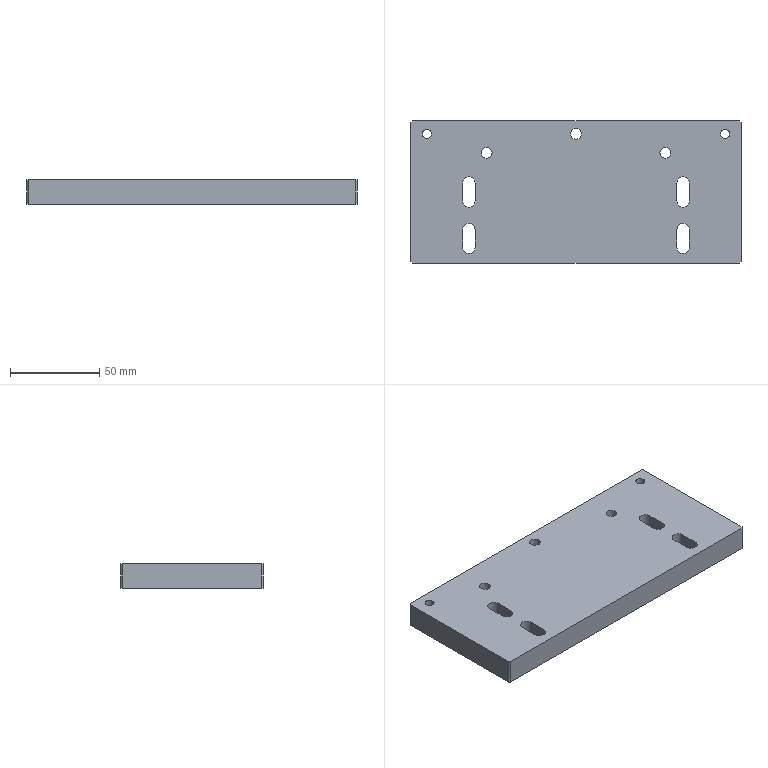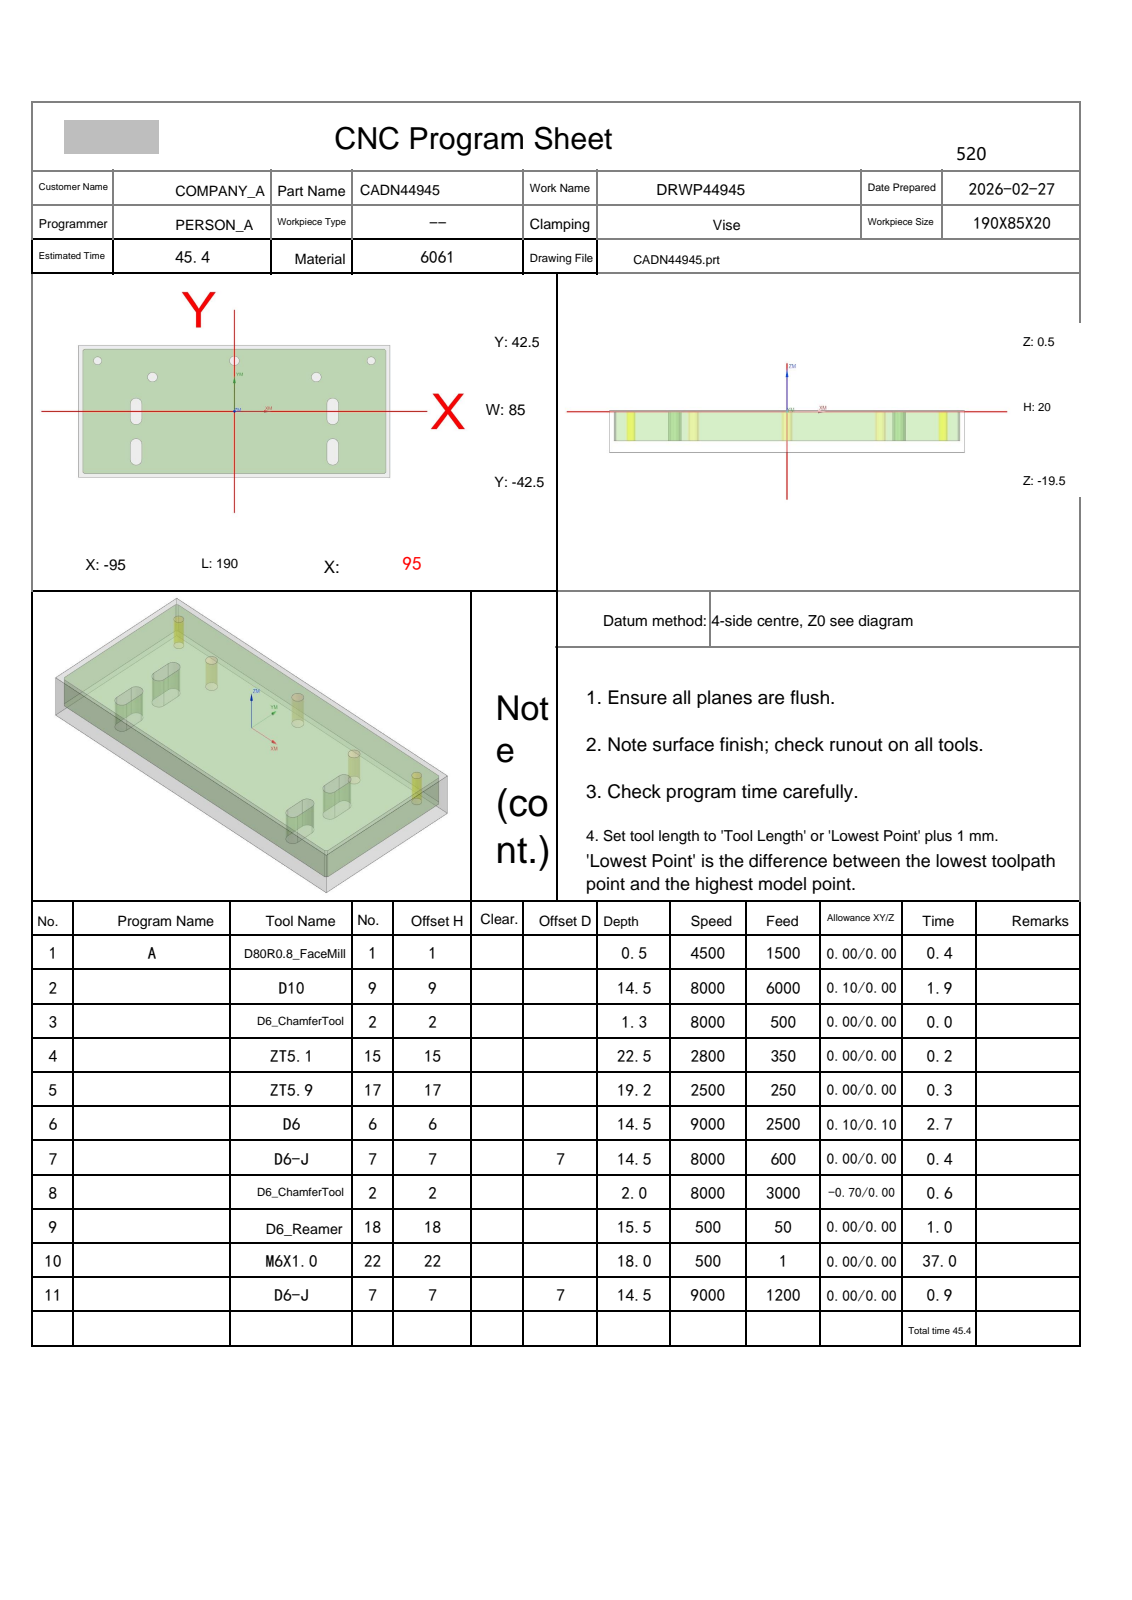NC program | NX | posted by the shop | part box 185 x 80 x 14 mm
Lines 439 to 1302 of 2772:
N6 T06 M06
(D6  D=6. R=0. H=06 ce=0.10 di=0.10)
G00 G90 G54 X-59.6 Y-26. M03 S9000
G43 H06 Z50.
M08
Z.5
G01 Y-21. Z.456 F2500.
G03 X-59.778 Y-20.667 Z.452 I-.4 J0.0
X-60. Y-20.6 Z.45 I-.222 J-.333
X-60.4 Y-21. Z.445 I0.0 J-.4
G01 Y-31. Z.357
G03 X-60. Y-31.4 Z.351 I.4 J0.0
X-59.6 Y-31. Z.345 I0.0 J.4
G01 Y-21. Z.257
G03 X-59.778 Y-20.667 Z.254 I-.4 J0.0
X-60. Y-20.6 Z.252 I-.222 J-.333
X-60.4 Y-21. Z.246 I0.0 J-.4
G01 Y-31. Z.158
G03 X-60. Y-31.4 Z.152 I.4 J0.0
X-59.6 Y-31. Z.147 I0.0 J.4
G01 Y-21. Z.059
G03 X-59.778 Y-20.667 Z.055 I-.4 J0.0
X-60. Y-20.6 Z.053 I-.222 J-.333
X-60.4 Y-21. Z.048 I0.0 J-.4
G01 Y-31. Z-.041
G03 X-60. Y-31.4 Z-.046 I.4 J0.0
X-59.6 Y-31. Z-.052 I0.0 J.4
G01 Y-21. Z-.14
G03 X-59.778 Y-20.667 Z-.143 I-.4 J0.0
X-60. Y-20.6 Z-.146 I-.222 J-.333
X-60.4 Y-21. Z-.151 I0.0 J-.4
G01 Y-31. Z-.239
G03 X-60. Y-31.4 Z-.245 I.4 J0.0
X-59.6 Y-31. Z-.25 I0.0 J.4
G01 Y-21. Z-.339
G03 X-59.778 Y-20.667 Z-.342 I-.4 J0.0
X-60. Y-20.6 Z-.344 I-.222 J-.333
X-60.4 Y-21. Z-.35 I0.0 J-.4
G01 Y-31. Z-.438
G03 X-60. Y-31.4 Z-.443 I.4 J0.0
X-59.6 Y-31. Z-.449 I0.0 J.4
G01 Y-21. Z-.537
G03 X-59.778 Y-20.667 Z-.541 I-.4 J0.0
X-60. Y-20.6 Z-.543 I-.222 J-.333
X-60.4 Y-21. Z-.548 I0.0 J-.4
G01 Y-31. Z-.637
G03 X-60. Y-31.4 Z-.642 I.4 J0.0
X-59.6 Y-31. Z-.648 I0.0 J.4
G01 Y-21. Z-.736
G03 X-59.778 Y-20.667 Z-.739 I-.4 J0.0
X-60. Y-20.6 Z-.741 I-.222 J-.333
X-60.4 Y-21. Z-.747 I0.0 J-.4
G01 Y-31. Z-.835
G03 X-60. Y-31.4 Z-.841 I.4 J0.0
X-59.6 Y-31. Z-.846 I0.0 J.4
G01 Y-21. Z-.935
G03 X-59.778 Y-20.667 Z-.938 I-.4 J0.0
X-60. Y-20.6 Z-.94 I-.222 J-.333
X-60.4 Y-21. Z-.946 I0.0 J-.4
G01 Y-31. Z-1.034
G03 X-60. Y-31.4 Z-1.039 I.4 J0.0
X-59.6 Y-31. Z-1.045 I0.0 J.4
G01 Y-21. Z-1.133
G03 X-59.778 Y-20.667 Z-1.137 I-.4 J0.0
X-60. Y-20.6 Z-1.139 I-.222 J-.333
X-60.4 Y-21. Z-1.144 I0.0 J-.4
G01 Y-31. Z-1.232
G03 X-60. Y-31.4 Z-1.238 I.4 J0.0
X-59.6 Y-31. Z-1.244 I0.0 J.4
G01 Y-21. Z-1.332
G03 X-59.778 Y-20.667 Z-1.335 I-.4 J0.0
X-60. Y-20.6 Z-1.337 I-.222 J-.333
X-60.4 Y-21. Z-1.343 I0.0 J-.4
G01 Y-31. Z-1.431
G03 X-60. Y-31.4 Z-1.437 I.4 J0.0
X-59.6 Y-31. Z-1.442 I0.0 J.4
G01 Y-21. Z-1.53
G03 X-59.778 Y-20.667 Z-1.534 I-.4 J0.0
X-60. Y-20.6 Z-1.536 I-.222 J-.333
X-60.4 Y-21. Z-1.542 I0.0 J-.4
G01 Y-31. Z-1.63
G03 X-60. Y-31.4 Z-1.635 I.4 J0.0
X-59.6 Y-31. Z-1.641 I0.0 J.4
G01 Y-21. Z-1.729
G03 X-59.778 Y-20.667 Z-1.733 I-.4 J0.0
X-60. Y-20.6 Z-1.735 I-.222 J-.333
X-60.4 Y-21. Z-1.74 I0.0 J-.4
G01 Y-31. Z-1.828
G03 X-60. Y-31.4 Z-1.834 I.4 J0.0
X-59.6 Y-31. Z-1.839 I0.0 J.4
G01 Y-21. Z-1.928
G03 X-59.778 Y-20.667 Z-1.931 I-.4 J0.0
X-60. Y-20.6 Z-1.933 I-.222 J-.333
X-60.4 Y-21. Z-1.939 I0.0 J-.4
G01 Y-31. Z-2.027
G03 X-60. Y-31.4 Z-2.033 I.4 J0.0
X-59.6 Y-31. Z-2.038 I0.0 J.4
G01 Y-21. Z-2.126
G03 X-59.778 Y-20.667 Z-2.13 I-.4 J0.0
X-60. Y-20.6 Z-2.132 I-.222 J-.333
X-60.4 Y-21. Z-2.137 I0.0 J-.4
G01 Y-31. Z-2.226
G03 X-60. Y-31.4 Z-2.231 I.4 J0.0
X-59.6 Y-31. Z-2.237 I0.0 J.4
G01 Y-21. Z-2.325
G03 X-59.778 Y-20.667 Z-2.328 I-.4 J0.0
X-60. Y-20.6 Z-2.33 I-.222 J-.333
X-60.4 Y-21. Z-2.336 I0.0 J-.4
G01 Y-31. Z-2.424
G03 X-60. Y-31.4 Z-2.43 I.4 J0.0
X-59.6 Y-31. Z-2.435 I0.0 J.4
G01 Y-21. Z-2.524
G03 X-59.778 Y-20.667 Z-2.527 I-.4 J0.0
X-60. Y-20.6 Z-2.529 I-.222 J-.333
X-60.4 Y-21. Z-2.535 I0.0 J-.4
G01 Y-31. Z-2.623
G03 X-60. Y-31.4 Z-2.628 I.4 J0.0
X-59.6 Y-31. Z-2.634 I0.0 J.4
G01 Y-21. Z-2.722
G03 X-59.778 Y-20.667 Z-2.726 I-.4 J0.0
X-60. Y-20.6 Z-2.728 I-.222 J-.333
X-60.4 Y-21. Z-2.733 I0.0 J-.4
G01 Y-31. Z-2.822
G03 X-60. Y-31.4 Z-2.827 I.4 J0.0
X-59.6 Y-31. Z-2.833 I0.0 J.4
G01 Y-21. Z-2.921
G03 X-59.778 Y-20.667 Z-2.924 I-.4 J0.0
X-60. Y-20.6 Z-2.926 I-.222 J-.333
X-60.4 Y-21. Z-2.932 I0.0 J-.4
G01 Y-31. Z-3.02
G03 X-60. Y-31.4 Z-3.026 I.4 J0.0
X-59.6 Y-31. Z-3.031 I0.0 J.4
G01 Y-21. Z-3.119
G03 X-59.778 Y-20.667 Z-3.123 I-.4 J0.0
X-60. Y-20.6 Z-3.125 I-.222 J-.333
X-60.4 Y-21. Z-3.131 I0.0 J-.4
G01 Y-31. Z-3.219
G03 X-60. Y-31.4 Z-3.224 I.4 J0.0
X-59.6 Y-31. Z-3.23 I0.0 J.4
G01 Y-21. Z-3.318
G03 X-59.778 Y-20.667 Z-3.322 I-.4 J0.0
X-60. Y-20.6 Z-3.324 I-.222 J-.333
X-60.4 Y-21. Z-3.329 I0.0 J-.4
G01 Y-31. Z-3.417
G03 X-60. Y-31.4 Z-3.423 I.4 J0.0
X-59.6 Y-31. Z-3.428 I0.0 J.4
G01 Y-21. Z-3.517
G03 X-59.778 Y-20.667 Z-3.52 I-.4 J0.0
X-60. Y-20.6 Z-3.522 I-.222 J-.333
X-60.4 Y-21. Z-3.528 I0.0 J-.4
G01 Y-31. Z-3.616
G03 X-60. Y-31.4 Z-3.622 I.4 J0.0
X-59.6 Y-31. Z-3.627 I0.0 J.4
G01 Y-21. Z-3.715
G03 X-59.778 Y-20.667 Z-3.719 I-.4 J0.0
X-60. Y-20.6 Z-3.721 I-.222 J-.333
X-60.4 Y-21. Z-3.726 I0.0 J-.4
G01 Y-31. Z-3.815
G03 X-60. Y-31.4 Z-3.82 I.4 J0.0
X-59.6 Y-31. Z-3.826 I0.0 J.4
G01 Y-21. Z-3.914
G03 X-59.778 Y-20.667 Z-3.917 I-.4 J0.0
X-60. Y-20.6 Z-3.92 I-.222 J-.333
X-60.4 Y-21. Z-3.925 I0.0 J-.4
G01 Y-31. Z-4.013
G03 X-60. Y-31.4 Z-4.019 I.4 J0.0
X-59.6 Y-31. Z-4.024 I0.0 J.4
G01 Y-21. Z-4.113
G03 X-59.778 Y-20.667 Z-4.116 I-.4 J0.0
X-60. Y-20.6 Z-4.118 I-.222 J-.333
X-60.4 Y-21. Z-4.124 I0.0 J-.4
G01 Y-31. Z-4.212
G03 X-60. Y-31.4 Z-4.217 I.4 J0.0
X-59.6 Y-31. Z-4.223 I0.0 J.4
G01 Y-21. Z-4.311
G03 X-59.778 Y-20.667 Z-4.315 I-.4 J0.0
X-60. Y-20.6 Z-4.317 I-.222 J-.333
X-60.4 Y-21. Z-4.322 I0.0 J-.4
G01 Y-31. Z-4.411
G03 X-60. Y-31.4 Z-4.416 I.4 J0.0
X-59.6 Y-31. Z-4.422 I0.0 J.4
G01 Y-21. Z-4.51
G03 X-59.778 Y-20.667 Z-4.513 I-.4 J0.0
X-60. Y-20.6 Z-4.515 I-.222 J-.333
X-60.4 Y-21. Z-4.521 I0.0 J-.4
G01 Y-31. Z-4.609
G03 X-60. Y-31.4 Z-4.615 I.4 J0.0
X-59.6 Y-31. Z-4.62 I0.0 J.4
G01 Y-21. Z-4.708
G03 X-59.778 Y-20.667 Z-4.712 I-.4 J0.0
X-60. Y-20.6 Z-4.714 I-.222 J-.333
X-60.4 Y-21. Z-4.72 I0.0 J-.4
G01 Y-31. Z-4.808
G03 X-60. Y-31.4 Z-4.813 I.4 J0.0
X-59.6 Y-31. Z-4.819 I0.0 J.4
G01 Y-21. Z-4.907
G03 X-59.778 Y-20.667 Z-4.911 I-.4 J0.0
X-60. Y-20.6 Z-4.913 I-.222 J-.333
X-60.4 Y-21. Z-4.918 I0.0 J-.4
G01 Y-31. Z-5.006
G03 X-60. Y-31.4 Z-5.012 I.4 J0.0
X-59.6 Y-31. Z-5.018 I0.0 J.4
G01 Y-21. Z-5.106
G03 X-59.778 Y-20.667 Z-5.109 I-.4 J0.0
X-60. Y-20.6 Z-5.111 I-.222 J-.333
X-60.4 Y-21. Z-5.117 I0.0 J-.4
G01 Y-31. Z-5.205
G03 X-60. Y-31.4 Z-5.211 I.4 J0.0
X-59.6 Y-31. Z-5.216 I0.0 J.4
G01 Y-21. Z-5.304
G03 X-59.778 Y-20.667 Z-5.308 I-.4 J0.0
X-60. Y-20.6 Z-5.31 I-.222 J-.333
X-60.4 Y-21. Z-5.315 I0.0 J-.4
G01 Y-31. Z-5.404
G03 X-60. Y-31.4 Z-5.409 I.4 J0.0
X-59.6 Y-31. Z-5.415 I0.0 J.4
G01 Y-21. Z-5.503
G03 X-59.778 Y-20.667 Z-5.506 I-.4 J0.0
X-60. Y-20.6 Z-5.509 I-.222 J-.333
X-60.4 Y-21. Z-5.514 I0.0 J-.4
G01 Y-31. Z-5.602
G03 X-60. Y-31.4 Z-5.608 I.4 J0.0
X-59.6 Y-31. Z-5.613 I0.0 J.4
G01 Y-21. Z-5.702
G03 X-59.778 Y-20.667 Z-5.705 I-.4 J0.0
X-60. Y-20.6 Z-5.707 I-.222 J-.333
X-60.4 Y-21. Z-5.713 I0.0 J-.4
G01 Y-31. Z-5.801
G03 X-60. Y-31.4 Z-5.807 I.4 J0.0
X-59.6 Y-31. Z-5.812 I0.0 J.4
G01 Y-21. Z-5.9
G03 X-59.778 Y-20.667 Z-5.904 I-.4 J0.0
X-60. Y-20.6 Z-5.906 I-.222 J-.333
X-60.4 Y-21. Z-5.911 I0.0 J-.4
G01 Y-31. Z-6.
G03 X-60. Y-31.4 Z-6.005 I.4 J0.0
X-59.6 Y-31. Z-6.011 I0.0 J.4
G01 Y-21. Z-6.099
G03 X-59.778 Y-20.667 Z-6.102 I-.4 J0.0
X-60. Y-20.6 Z-6.104 I-.222 J-.333
X-60.4 Y-21. Z-6.11 I0.0 J-.4
G01 Y-31. Z-6.198
G03 X-60. Y-31.4 Z-6.204 I.4 J0.0
X-59.6 Y-31. Z-6.209 I0.0 J.4
G01 Y-21. Z-6.298
G03 X-59.778 Y-20.667 Z-6.301 I-.4 J0.0
X-60. Y-20.6 Z-6.303 I-.222 J-.333
X-60.4 Y-21. Z-6.309 I0.0 J-.4
G01 Y-31. Z-6.397
G03 X-60. Y-31.4 Z-6.402 I.4 J0.0
X-59.6 Y-31. Z-6.408 I0.0 J.4
G01 Y-21. Z-6.496
G03 X-59.778 Y-20.667 Z-6.5 I-.4 J0.0
X-60. Y-20.6 Z-6.502 I-.222 J-.333
X-60.4 Y-21. Z-6.507 I0.0 J-.4
G01 Y-31. Z-6.595
G03 X-60. Y-31.4 Z-6.601 I.4 J0.0
X-59.6 Y-31. Z-6.607 I0.0 J.4
G01 Y-21. Z-6.695
G03 X-59.778 Y-20.667 Z-6.698 I-.4 J0.0
X-60. Y-20.6 Z-6.7 I-.222 J-.333
X-60.4 Y-21. Z-6.706 I0.0 J-.4
G01 Y-31. Z-6.794
G03 X-60. Y-31.4 Z-6.8 I.4 J0.0
X-59.6 Y-31. Z-6.805 I0.0 J.4
G01 Y-21. Z-6.893
G03 X-59.778 Y-20.667 Z-6.897 I-.4 J0.0
X-60. Y-20.6 Z-6.899 I-.222 J-.333
X-60.4 Y-21. Z-6.905 I0.0 J-.4
G01 Y-31. Z-6.993
G03 X-60. Y-31.4 Z-6.998 I.4 J0.0
X-59.6 Y-31. Z-7.004 I0.0 J.4
G01 Y-21. Z-7.092
G03 X-59.778 Y-20.667 Z-7.096 I-.4 J0.0
X-60. Y-20.6 Z-7.098 I-.222 J-.333
X-60.4 Y-21. Z-7.103 I0.0 J-.4
G01 Y-31. Z-7.191
G03 X-60. Y-31.4 Z-7.197 I.4 J0.0
X-59.6 Y-31. Z-7.202 I0.0 J.4
G01 Y-21. Z-7.291
G03 X-59.778 Y-20.667 Z-7.294 I-.4 J0.0
X-60. Y-20.6 Z-7.296 I-.222 J-.333
X-60.4 Y-21. Z-7.302 I0.0 J-.4
G01 Y-31. Z-7.39
G03 X-60. Y-31.4 Z-7.396 I.4 J0.0
X-59.6 Y-31. Z-7.401 I0.0 J.4
G01 Y-21. Z-7.489
G03 X-59.778 Y-20.667 Z-7.493 I-.4 J0.0
X-60. Y-20.6 Z-7.495 I-.222 J-.333
X-60.4 Y-21. Z-7.5 I0.0 J-.4
G01 Y-31. Z-7.589
G03 X-60. Y-31.4 Z-7.594 I.4 J0.0
X-59.6 Y-31. Z-7.6 I0.0 J.4
G01 Y-21. Z-7.688
G03 X-59.778 Y-20.667 Z-7.691 I-.4 J0.0
X-60. Y-20.6 Z-7.693 I-.222 J-.333
X-60.4 Y-21. Z-7.699 I0.0 J-.4
G01 Y-31. Z-7.787
G03 X-60. Y-31.4 Z-7.793 I.4 J0.0
X-59.6 Y-31. Z-7.798 I0.0 J.4
G01 Y-21. Z-7.887
G03 X-59.778 Y-20.667 Z-7.89 I-.4 J0.0
X-60. Y-20.6 Z-7.892 I-.222 J-.333
X-60.4 Y-21. Z-7.898 I0.0 J-.4
G01 Y-31. Z-7.986
G03 X-60. Y-31.4 Z-7.991 I.4 J0.0
X-59.6 Y-31. Z-7.997 I0.0 J.4
G01 Y-21. Z-8.085
G03 X-59.778 Y-20.667 Z-8.089 I-.4 J0.0
X-60. Y-20.6 Z-8.091 I-.222 J-.333
X-60.4 Y-21. Z-8.096 I0.0 J-.4
G01 Y-31. Z-8.185
G03 X-60. Y-31.4 Z-8.19 I.4 J0.0
X-59.6 Y-31. Z-8.196 I0.0 J.4
G01 Y-21. Z-8.284
G03 X-59.778 Y-20.667 Z-8.287 I-.4 J0.0
X-60. Y-20.6 Z-8.289 I-.222 J-.333
X-60.4 Y-21. Z-8.295 I0.0 J-.4
G01 Y-31. Z-8.383
G03 X-60. Y-31.4 Z-8.389 I.4 J0.0
X-59.6 Y-31. Z-8.394 I0.0 J.4
G01 Y-21. Z-8.482
G03 X-59.778 Y-20.667 Z-8.486 I-.4 J0.0
X-60. Y-20.6 Z-8.488 I-.222 J-.333
X-60.4 Y-21. Z-8.494 I0.0 J-.4
G01 Y-31. Z-8.582
G03 X-60. Y-31.4 Z-8.587 I.4 J0.0
X-59.6 Y-31. Z-8.593 I0.0 J.4
G01 Y-21. Z-8.681
G03 X-59.778 Y-20.667 Z-8.685 I-.4 J0.0
X-60. Y-20.6 Z-8.687 I-.222 J-.333
X-60.4 Y-21. Z-8.692 I0.0 J-.4
G01 Y-31. Z-8.78
G03 X-60. Y-31.4 Z-8.786 I.4 J0.0
X-59.6 Y-31. Z-8.792 I0.0 J.4
G01 Y-21. Z-8.88
G03 X-59.778 Y-20.667 Z-8.883 I-.4 J0.0
X-60. Y-20.6 Z-8.885 I-.222 J-.333
X-60.4 Y-21. Z-8.891 I0.0 J-.4
G01 Y-31. Z-8.979
G03 X-60. Y-31.4 Z-8.985 I.4 J0.0
X-59.6 Y-31. Z-8.99 I0.0 J.4
G01 Y-21. Z-9.078
G03 X-59.778 Y-20.667 Z-9.082 I-.4 J0.0
X-60. Y-20.6 Z-9.084 I-.222 J-.333
X-60.4 Y-21. Z-9.089 I0.0 J-.4
G01 Y-31. Z-9.178
G03 X-60. Y-31.4 Z-9.183 I.4 J0.0
X-59.6 Y-31. Z-9.189 I0.0 J.4
G01 Y-21. Z-9.277
G03 X-59.778 Y-20.667 Z-9.28 I-.4 J0.0
X-60. Y-20.6 Z-9.283 I-.222 J-.333
X-60.4 Y-21. Z-9.288 I0.0 J-.4
G01 Y-31. Z-9.376
G03 X-60. Y-31.4 Z-9.382 I.4 J0.0
X-59.6 Y-31. Z-9.387 I0.0 J.4
G01 Y-21. Z-9.476
G03 X-59.778 Y-20.667 Z-9.479 I-.4 J0.0
X-60. Y-20.6 Z-9.481 I-.222 J-.333
X-60.4 Y-21. Z-9.487 I0.0 J-.4
G01 Y-31. Z-9.575
G03 X-60. Y-31.4 Z-9.58 I.4 J0.0
X-59.6 Y-31. Z-9.586 I0.0 J.4
G01 Y-21. Z-9.674
G03 X-59.778 Y-20.667 Z-9.678 I-.4 J0.0
X-60. Y-20.6 Z-9.68 I-.222 J-.333
X-60.4 Y-21. Z-9.685 I0.0 J-.4
G01 Y-31. Z-9.774
G03 X-60. Y-31.4 Z-9.779 I.4 J0.0
X-59.6 Y-31. Z-9.785 I0.0 J.4
G01 Y-21. Z-9.873
G03 X-59.778 Y-20.667 Z-9.876 I-.4 J0.0
X-60. Y-20.6 Z-9.878 I-.222 J-.333
X-60.4 Y-21. Z-9.884 I0.0 J-.4
G01 Y-31. Z-9.972
G03 X-60. Y-31.4 Z-9.978 I.4 J0.0
X-59.6 Y-31. Z-9.983 I0.0 J.4
G01 Y-21. Z-10.072
G03 X-59.778 Y-20.667 Z-10.075 I-.4 J0.0
X-60. Y-20.6 Z-10.077 I-.222 J-.333
X-60.4 Y-21. Z-10.083 I0.0 J-.4
G01 Y-31. Z-10.171
G03 X-60. Y-31.4 Z-10.176 I.4 J0.0
X-59.6 Y-31. Z-10.182 I0.0 J.4
G01 Y-21. Z-10.27
G03 X-59.778 Y-20.667 Z-10.274 I-.4 J0.0
X-60. Y-20.6 Z-10.276 I-.222 J-.333
X-60.4 Y-21. Z-10.281 I0.0 J-.4
G01 Y-31. Z-10.369
G03 X-60. Y-31.4 Z-10.375 I.4 J0.0
X-59.6 Y-31. Z-10.381 I0.0 J.4
G01 Y-21. Z-10.469
G03 X-59.778 Y-20.667 Z-10.472 I-.4 J0.0
X-60. Y-20.6 Z-10.474 I-.222 J-.333
X-60.4 Y-21. Z-10.48 I0.0 J-.4
G01 Y-31. Z-10.568
G03 X-60. Y-31.4 Z-10.574 I.4 J0.0
X-59.6 Y-31. Z-10.579 I0.0 J.4
G01 Y-21. Z-10.667
G03 X-59.778 Y-20.667 Z-10.671 I-.4 J0.0
X-60. Y-20.6 Z-10.673 I-.222 J-.333
X-60.4 Y-21. Z-10.678 I0.0 J-.4
G01 Y-31. Z-10.767
G03 X-60. Y-31.4 Z-10.772 I.4 J0.0
X-59.6 Y-31. Z-10.778 I0.0 J.4
G01 Y-21. Z-10.866
G03 X-59.778 Y-20.667 Z-10.87 I-.4 J0.0
X-60. Y-20.6 Z-10.872 I-.222 J-.333
X-60.4 Y-21. Z-10.877 I0.0 J-.4
G01 Y-31. Z-10.965
G03 X-60. Y-31.4 Z-10.971 I.4 J0.0
X-59.6 Y-31. Z-10.976 I0.0 J.4
G01 Y-21. Z-11.065
G03 X-59.778 Y-20.667 Z-11.068 I-.4 J0.0
X-60. Y-20.6 Z-11.07 I-.222 J-.333
X-60.4 Y-21. Z-11.076 I0.0 J-.4
G01 Y-31. Z-11.164
G03 X-60. Y-31.4 Z-11.17 I.4 J0.0
X-59.6 Y-31. Z-11.175 I0.0 J.4
G01 Y-21. Z-11.263
G03 X-59.778 Y-20.667 Z-11.267 I-.4 J0.0
X-60. Y-20.6 Z-11.269 I-.222 J-.333
X-60.4 Y-21. Z-11.274 I0.0 J-.4
G01 Y-31. Z-11.363
G03 X-60. Y-31.4 Z-11.368 I.4 J0.0
X-59.6 Y-31. Z-11.374 I0.0 J.4
G01 Y-21. Z-11.462
G03 X-59.778 Y-20.667 Z-11.465 I-.4 J0.0
X-60. Y-20.6 Z-11.467 I-.222 J-.333
X-60.4 Y-21. Z-11.473 I0.0 J-.4
G01 Y-31. Z-11.561
G03 X-60. Y-31.4 Z-11.567 I.4 J0.0
X-59.6 Y-31. Z-11.572 I0.0 J.4
G01 Y-21. Z-11.661
G03 X-59.778 Y-20.667 Z-11.664 I-.4 J0.0
X-60. Y-20.6 Z-11.666 I-.222 J-.333
X-60.4 Y-21. Z-11.672 I0.0 J-.4
G01 Y-31. Z-11.76
G03 X-60. Y-31.4 Z-11.765 I.4 J0.0
X-59.6 Y-31. Z-11.771 I0.0 J.4
G01 Y-21. Z-11.859
G03 X-59.778 Y-20.667 Z-11.863 I-.4 J0.0
X-60. Y-20.6 Z-11.865 I-.222 J-.333
X-60.4 Y-21. Z-11.87 I0.0 J-.4
G01 Y-31. Z-11.958
G03 X-60. Y-31.4 Z-11.964 I.4 J0.0
X-59.6 Y-31. Z-11.97 I0.0 J.4
G01 Y-21. Z-12.058
G03 X-59.778 Y-20.667 Z-12.061 I-.4 J0.0
X-60. Y-20.6 Z-12.063 I-.222 J-.333
X-60.4 Y-21. Z-12.069 I0.0 J-.4
G01 Y-31. Z-12.157
G03 X-60. Y-31.4 Z-12.163 I.4 J0.0
X-59.6 Y-31. Z-12.168 I0.0 J.4
G01 Y-21. Z-12.256
G03 X-59.778 Y-20.667 Z-12.26 I-.4 J0.0
X-60. Y-20.6 Z-12.262 I-.222 J-.333
X-60.4 Y-21. Z-12.268 I0.0 J-.4
G01 Y-31. Z-12.356
G03 X-60. Y-31.4 Z-12.361 I.4 J0.0
X-59.6 Y-31. Z-12.367 I0.0 J.4
G01 Y-21. Z-12.455
G03 X-59.778 Y-20.667 Z-12.459 I-.4 J0.0
X-60. Y-20.6 Z-12.461 I-.222 J-.333
X-60.4 Y-21. Z-12.466 I0.0 J-.4
G01 Y-31. Z-12.554
G03 X-60. Y-31.4 Z-12.56 I.4 J0.0
X-59.6 Y-31. Z-12.565 I0.0 J.4
G01 Y-21. Z-12.654
G03 X-59.778 Y-20.667 Z-12.657 I-.4 J0.0
X-60. Y-20.6 Z-12.659 I-.222 J-.333
X-60.4 Y-21. Z-12.665 I0.0 J-.4
G01 Y-31. Z-12.753
G03 X-60. Y-31.4 Z-12.759 I.4 J0.0
X-59.6 Y-31. Z-12.764 I0.0 J.4
G01 Y-21. Z-12.852
G03 X-59.778 Y-20.667 Z-12.856 I-.4 J0.0
X-60. Y-20.6 Z-12.858 I-.222 J-.333
X-60.4 Y-21. Z-12.863 I0.0 J-.4
G01 Y-31. Z-12.952
G03 X-60. Y-31.4 Z-12.957 I.4 J0.0
X-59.6 Y-31. Z-12.963 I0.0 J.4
G01 Y-21. Z-13.051
G03 X-59.778 Y-20.667 Z-13.054 I-.4 J0.0
X-60. Y-20.6 Z-13.057 I-.222 J-.333
X-60.4 Y-21. Z-13.062 I0.0 J-.4
G01 Y-31. Z-13.15
G03 X-60. Y-31.4 Z-13.156 I.4 J0.0
X-59.6 Y-31. Z-13.161 I0.0 J.4
G01 Y-21. Z-13.25
G03 X-59.778 Y-20.667 Z-13.253 I-.4 J0.0
X-60. Y-20.6 Z-13.255 I-.222 J-.333
X-60.4 Y-21. Z-13.261 I0.0 J-.4
G01 Y-31. Z-13.349
G03 X-60. Y-31.4 Z-13.354 I.4 J0.0
X-59.6 Y-31. Z-13.36 I0.0 J.4
G01 Y-21. Z-13.448
G03 X-59.778 Y-20.667 Z-13.452 I-.4 J0.0
X-60. Y-20.6 Z-13.454 I-.222 J-.333
X-60.4 Y-21. Z-13.459 I0.0 J-.4
G01 Y-31. Z-13.548
G03 X-60. Y-31.4 Z-13.553 I.4 J0.0
X-59.6 Y-31. Z-13.559 I0.0 J.4
G01 Y-21. Z-13.647
G03 X-59.778 Y-20.667 Z-13.65 I-.4 J0.0
X-60. Y-20.6 Z-13.652 I-.222 J-.333
X-60.4 Y-21. Z-13.658 I0.0 J-.4
G01 Y-31. Z-13.746
G03 X-60. Y-31.4 Z-13.752 I.4 J0.0
X-59.6 Y-31. Z-13.757 I0.0 J.4
G01 Y-21. Z-13.845
G03 X-59.778 Y-20.667 Z-13.849 I-.4 J0.0
X-60. Y-20.6 Z-13.851 I-.222 J-.333
X-60.4 Y-21. Z-13.857 I0.0 J-.4
G01 Y-31. Z-13.945
G03 X-60. Y-31.4 Z-13.95 I.4 J0.0
X-59.6 Y-31. Z-13.956 I0.0 J.4
G01 Y-26. Z-14.
Y-21.
G03 X-60. Y-20.6 I-.4 J0.0
X-60.4 Y-21. I0.0 J-.4
G01 Y-31.
G03 X-60. Y-31.4 I.4 J0.0
X-59.6 Y-31. I0.0 J.4
G01 Y-26.
Y-25.5
Z-13.
G00 Z50.
Y0.0
Z.5
G01 Y5. Z.456
G03 X-60. Y5.4 Z.45 I-.4 J0.0
X-60.4 Y5. Z.445 I0.0 J-.4
G01 Y-5. Z.357
G03 X-60. Y-5.4 Z.351 I.4 J0.0
X-59.6 Y-5. Z.345 I0.0 J.4
G01 Y5. Z.257
G03 X-60. Y5.4 Z.252 I-.4 J0.0
X-60.4 Y5. Z.246 I0.0 J-.4
G01 Y-5. Z.158
G03 X-60. Y-5.4 Z.152 I.4 J0.0
X-59.6 Y-5. Z.147 I0.0 J.4
G01 Y5. Z.059
G03 X-60. Y5.4 Z.053 I-.4 J0.0
X-60.4 Y5. Z.048 I0.0 J-.4
G01 Y-5. Z-.041
G03 X-60. Y-5.4 Z-.046 I.4 J0.0
X-59.6 Y-5. Z-.052 I0.0 J.4
G01 Y5. Z-.14
G03 X-60. Y5.4 Z-.146 I-.4 J0.0
X-60.4 Y5. Z-.151 I0.0 J-.4
G01 Y-5. Z-.239
G03 X-60. Y-5.4 Z-.245 I.4 J0.0
X-59.6 Y-5. Z-.25 I0.0 J.4
G01 Y5. Z-.339
G03 X-60. Y5.4 Z-.344 I-.4 J0.0
X-60.4 Y5. Z-.35 I0.0 J-.4
G01 Y-5. Z-.438
G03 X-60. Y-5.4 Z-.443 I.4 J0.0
X-59.6 Y-5. Z-.449 I0.0 J.4
G01 Y5. Z-.537
G03 X-60. Y5.4 Z-.543 I-.4 J0.0
X-60.4 Y5. Z-.548 I0.0 J-.4
G01 Y-5. Z-.637
G03 X-60. Y-5.4 Z-.642 I.4 J0.0
X-59.6 Y-5. Z-.648 I0.0 J.4
G01 Y5. Z-.736
G03 X-60. Y5.4 Z-.741 I-.4 J0.0
X-60.4 Y5. Z-.747 I0.0 J-.4
G01 Y-5. Z-.835
G03 X-60. Y-5.4 Z-.841 I.4 J0.0
X-59.6 Y-5. Z-.846 I0.0 J.4
G01 Y5. Z-.935
G03 X-60. Y5.4 Z-.94 I-.4 J0.0
X-60.4 Y5. Z-.946 I0.0 J-.4
G01 Y-5. Z-1.034
G03 X-60. Y-5.4 Z-1.039 I.4 J0.0
X-59.6 Y-5. Z-1.045 I0.0 J.4
G01 Y5. Z-1.133
G03 X-60. Y5.4 Z-1.139 I-.4 J0.0
X-60.4 Y5. Z-1.144 I0.0 J-.4
G01 Y-5. Z-1.232
G03 X-60. Y-5.4 Z-1.238 I.4 J0.0
X-59.6 Y-5. Z-1.244 I0.0 J.4
G01 Y5. Z-1.332
G03 X-60. Y5.4 Z-1.337 I-.4 J0.0
X-60.4 Y5. Z-1.343 I0.0 J-.4
G01 Y-5. Z-1.431
G03 X-60. Y-5.4 Z-1.437 I.4 J0.0
X-59.6 Y-5. Z-1.442 I0.0 J.4
G01 Y5. Z-1.53
G03 X-60. Y5.4 Z-1.536 I-.4 J0.0
X-60.4 Y5. Z-1.542 I0.0 J-.4
G01 Y-5. Z-1.63
G03 X-60. Y-5.4 Z-1.635 I.4 J0.0
X-59.6 Y-5. Z-1.641 I0.0 J.4
G01 Y5. Z-1.729
G03 X-60. Y5.4 Z-1.735 I-.4 J0.0
X-60.4 Y5. Z-1.74 I0.0 J-.4
G01 Y-5. Z-1.828
G03 X-60. Y-5.4 Z-1.834 I.4 J0.0
X-59.6 Y-5. Z-1.839 I0.0 J.4
G01 Y5. Z-1.928
G03 X-60. Y5.4 Z-1.933 I-.4 J0.0
X-60.4 Y5. Z-1.939 I0.0 J-.4
G01 Y-5. Z-2.027
G03 X-60. Y-5.4 Z-2.033 I.4 J0.0
X-59.6 Y-5. Z-2.038 I0.0 J.4
G01 Y5. Z-2.126
G03 X-60. Y5.4 Z-2.132 I-.4 J0.0
X-60.4 Y5. Z-2.137 I0.0 J-.4
G01 Y-5. Z-2.226
G03 X-60. Y-5.4 Z-2.231 I.4 J0.0
X-59.6 Y-5. Z-2.237 I0.0 J.4
G01 Y5. Z-2.325
G03 X-60. Y5.4 Z-2.33 I-.4 J0.0
X-60.4 Y5. Z-2.336 I0.0 J-.4
G01 Y-5. Z-2.424
G03 X-60. Y-5.4 Z-2.43 I.4 J0.0
X-59.6 Y-5. Z-2.435 I0.0 J.4
G01 Y5. Z-2.524
G03 X-60. Y5.4 Z-2.529 I-.4 J0.0
X-60.4 Y5. Z-2.535 I0.0 J-.4
G01 Y-5. Z-2.623
G03 X-60. Y-5.4 Z-2.628 I.4 J0.0
X-59.6 Y-5. Z-2.634 I0.0 J.4
G01 Y5. Z-2.722
G03 X-60. Y5.4 Z-2.728 I-.4 J0.0
X-60.4 Y5. Z-2.733 I0.0 J-.4
G01 Y-5. Z-2.822
G03 X-60. Y-5.4 Z-2.827 I.4 J0.0
X-59.6 Y-5. Z-2.833 I0.0 J.4
G01 Y5. Z-2.921
G03 X-60. Y5.4 Z-2.926 I-.4 J0.0
X-60.4 Y5. Z-2.932 I0.0 J-.4
G01 Y-5. Z-3.02
G03 X-60. Y-5.4 Z-3.026 I.4 J0.0
X-59.6 Y-5. Z-3.031 I0.0 J.4
G01 Y5. Z-3.119
G03 X-60. Y5.4 Z-3.125 I-.4 J0.0
X-60.4 Y5. Z-3.131 I0.0 J-.4
G01 Y-5. Z-3.219
G03 X-60. Y-5.4 Z-3.224 I.4 J0.0
X-59.6 Y-5. Z-3.23 I0.0 J.4
G01 Y5. Z-3.318
G03 X-60. Y5.4 Z-3.324 I-.4 J0.0
X-60.4 Y5. Z-3.329 I0.0 J-.4
G01 Y-5. Z-3.417
G03 X-60. Y-5.4 Z-3.423 I.4 J0.0
X-59.6 Y-5. Z-3.428 I0.0 J.4
G01 Y5. Z-3.517
G03 X-60. Y5.4 Z-3.522 I-.4 J0.0
X-60.4 Y5. Z-3.528 I0.0 J-.4
G01 Y-5. Z-3.616
G03 X-60. Y-5.4 Z-3.622 I.4 J0.0
X-59.6 Y-5. Z-3.627 I0.0 J.4
G01 Y5. Z-3.715
G03 X-60. Y5.4 Z-3.721 I-.4 J0.0
X-60.4 Y5. Z-3.726 I0.0 J-.4
G01 Y-5. Z-3.815
G03 X-60. Y-5.4 Z-3.82 I.4 J0.0
X-59.6 Y-5. Z-3.826 I0.0 J.4
G01 Y5. Z-3.914
G03 X-60. Y5.4 Z-3.92 I-.4 J0.0
X-60.4 Y5. Z-3.925 I0.0 J-.4
G01 Y-5. Z-4.013
G03 X-60. Y-5.4 Z-4.019 I.4 J0.0
X-59.6 Y-5. Z-4.024 I0.0 J.4
G01 Y5. Z-4.113
G03 X-60. Y5.4 Z-4.118 I-.4 J0.0
X-60.4 Y5. Z-4.124 I0.0 J-.4
G01 Y-5. Z-4.212
G03 X-60. Y-5.4 Z-4.217 I.4 J0.0
X-59.6 Y-5. Z-4.223 I0.0 J.4
G01 Y5. Z-4.311
G03 X-60. Y5.4 Z-4.317 I-.4 J0.0
X-60.4 Y5. Z-4.322 I0.0 J-.4
G01 Y-5. Z-4.411
G03 X-60. Y-5.4 Z-4.416 I.4 J0.0
X-59.6 Y-5. Z-4.422 I0.0 J.4
G01 Y5. Z-4.51
G03 X-60. Y5.4 Z-4.515 I-.4 J0.0
X-60.4 Y5. Z-4.521 I0.0 J-.4
G01 Y-5. Z-4.609
G03 X-60. Y-5.4 Z-4.615 I.4 J0.0
X-59.6 Y-5. Z-4.62 I0.0 J.4
G01 Y5. Z-4.708
G03 X-60. Y5.4 Z-4.714 I-.4 J0.0
X-60.4 Y5. Z-4.72 I0.0 J-.4
G01 Y-5. Z-4.808
G03 X-60. Y-5.4 Z-4.813 I.4 J0.0
X-59.6 Y-5. Z-4.819 I0.0 J.4
G01 Y5. Z-4.907
G03 X-60. Y5.4 Z-4.913 I-.4 J0.0
X-60.4 Y5. Z-4.918 I0.0 J-.4
G01 Y-5. Z-5.006
G03 X-60. Y-5.4 Z-5.012 I.4 J0.0
X-59.6 Y-5. Z-5.018 I0.0 J.4
G01 Y5. Z-5.106
G03 X-60. Y5.4 Z-5.111 I-.4 J0.0
X-60.4 Y5. Z-5.117 I0.0 J-.4
G01 Y-5. Z-5.205
G03 X-60. Y-5.4 Z-5.211 I.4 J0.0
X-59.6 Y-5. Z-5.216 I0.0 J.4
G01 Y5. Z-5.304
G03 X-60. Y5.4 Z-5.31 I-.4 J0.0
X-60.4 Y5. Z-5.315 I0.0 J-.4
G01 Y-5. Z-5.404
G03 X-60. Y-5.4 Z-5.409 I.4 J0.0
X-59.6 Y-5. Z-5.415 I0.0 J.4
G01 Y5. Z-5.503
G03 X-60. Y5.4 Z-5.509 I-.4 J0.0
X-60.4 Y5. Z-5.514 I0.0 J-.4
G01 Y-5. Z-5.602
G03 X-60. Y-5.4 Z-5.608 I.4 J0.0
X-59.6 Y-5. Z-5.613 I0.0 J.4
G01 Y5. Z-5.702
G03 X-60. Y5.4 Z-5.707 I-.4 J0.0
X-60.4 Y5. Z-5.713 I0.0 J-.4
G01 Y-5. Z-5.801
G03 X-60. Y-5.4 Z-5.807 I.4 J0.0
X-59.6 Y-5. Z-5.812 I0.0 J.4
G01 Y5. Z-5.9
G03 X-60. Y5.4 Z-5.906 I-.4 J0.0
X-60.4 Y5. Z-5.911 I0.0 J-.4
G01 Y-5. Z-6.
G03 X-60. Y-5.4 Z-6.005 I.4 J0.0
X-59.6 Y-5. Z-6.011 I0.0 J.4
G01 Y5. Z-6.099
G03 X-60. Y5.4 Z-6.104 I-.4 J0.0
X-60.4 Y5. Z-6.11 I0.0 J-.4
G01 Y-5. Z-6.198
G03 X-60. Y-5.4 Z-6.204 I.4 J0.0
X-59.6 Y-5. Z-6.209 I0.0 J.4
G01 Y5. Z-6.298
G03 X-60. Y5.4 Z-6.303 I-.4 J0.0
X-60.4 Y5. Z-6.309 I0.0 J-.4
G01 Y-5. Z-6.397
G03 X-60. Y-5.4 Z-6.402 I.4 J0.0
X-59.6 Y-5. Z-6.408 I0.0 J.4
G01 Y5. Z-6.496
G03 X-60. Y5.4 Z-6.502 I-.4 J0.0
X-60.4 Y5. Z-6.507 I0.0 J-.4
G01 Y-5. Z-6.595
G03 X-60. Y-5.4 Z-6.601 I.4 J0.0
X-59.6 Y-5. Z-6.607 I0.0 J.4
G01 Y5. Z-6.695
G03 X-60. Y5.4 Z-6.7 I-.4 J0.0
X-60.4 Y5. Z-6.706 I0.0 J-.4
G01 Y-5. Z-6.794
G03 X-60. Y-5.4 Z-6.8 I.4 J0.0
X-59.6 Y-5. Z-6.805 I0.0 J.4
G01 Y5. Z-6.893
G03 X-60. Y5.4 Z-6.899 I-.4 J0.0
X-60.4 Y5. Z-6.905 I0.0 J-.4
G01 Y-5. Z-6.993
G03 X-60. Y-5.4 Z-6.998 I.4 J0.0
X-59.6 Y-5. Z-7.004 I0.0 J.4
G01 Y5. Z-7.092
G03 X-60. Y5.4 Z-7.098 I-.4 J0.0
X-60.4 Y5. Z-7.103 I0.0 J-.4
G01 Y-5. Z-7.191
G03 X-60. Y-5.4 Z-7.197 I.4 J0.0
X-59.6 Y-5. Z-7.202 I0.0 J.4
G01 Y5. Z-7.291
G03 X-60. Y5.4 Z-7.296 I-.4 J0.0
X-60.4 Y5. Z-7.302 I0.0 J-.4
G01 Y-5. Z-7.39
G03 X-60. Y-5.4 Z-7.396 I.4 J0.0
X-59.6 Y-5. Z-7.401 I0.0 J.4
G01 Y5. Z-7.489
G03 X-60. Y5.4 Z-7.495 I-.4 J0.0
X-60.4 Y5. Z-7.5 I0.0 J-.4
G01 Y-5. Z-7.589
G03 X-60. Y-5.4 Z-7.594 I.4 J0.0
X-59.6 Y-5. Z-7.6 I0.0 J.4
G01 Y5. Z-7.688
G03 X-60. Y5.4 Z-7.693 I-.4 J0.0
X-60.4 Y5. Z-7.699 I0.0 J-.4
G01 Y-5. Z-7.787
G03 X-60. Y-5.4 Z-7.793 I.4 J0.0
X-59.6 Y-5. Z-7.798 I0.0 J.4
G01 Y5. Z-7.887
G03 X-60. Y5.4 Z-7.892 I-.4 J0.0
X-60.4 Y5. Z-7.898 I0.0 J-.4
G01 Y-5. Z-7.986
G03 X-60. Y-5.4 Z-7.991 I.4 J0.0
X-59.6 Y-5. Z-7.997 I0.0 J.4
G01 Y5. Z-8.085
G03 X-60. Y5.4 Z-8.091 I-.4 J0.0
X-60.4 Y5. Z-8.096 I0.0 J-.4
G01 Y-5. Z-8.185
G03 X-60. Y-5.4 Z-8.19 I.4 J0.0
X-59.6 Y-5. Z-8.196 I0.0 J.4
G01 Y5. Z-8.284
G03 X-60. Y5.4 Z-8.289 I-.4 J0.0
X-60.4 Y5. Z-8.295 I0.0 J-.4
G01 Y-5. Z-8.383
G03 X-60. Y-5.4 Z-8.389 I.4 J0.0
X-59.6 Y-5. Z-8.394 I0.0 J.4
G01 Y5. Z-8.482
G03 X-60. Y5.4 Z-8.488 I-.4 J0.0
X-60.4 Y5. Z-8.494 I0.0 J-.4
G01 Y-5. Z-8.582
G03 X-60. Y-5.4 Z-8.587 I.4 J0.0
X-59.6 Y-5. Z-8.593 I0.0 J.4
G01 Y5. Z-8.681
G03 X-60. Y5.4 Z-8.687 I-.4 J0.0
X-60.4 Y5. Z-8.692 I0.0 J-.4
G01 Y-5. Z-8.78
G03 X-60. Y-5.4 Z-8.786 I.4 J0.0
X-59.6 Y-5. Z-8.792 I0.0 J.4
G01 Y5. Z-8.88
G03 X-60. Y5.4 Z-8.885 I-.4 J0.0
X-60.4 Y5. Z-8.891 I0.0 J-.4
G01 Y-5. Z-8.979
G03 X-60. Y-5.4 Z-8.985 I.4 J0.0
X-59.6 Y-5. Z-8.99 I0.0 J.4
G01 Y5. Z-9.078
G03 X-60. Y5.4 Z-9.084 I-.4 J0.0
X-60.4 Y5. Z-9.089 I0.0 J-.4
G01 Y-5. Z-9.178
G03 X-60. Y-5.4 Z-9.183 I.4 J0.0
X-59.6 Y-5. Z-9.189 I0.0 J.4
G01 Y5. Z-9.277
G03 X-60. Y5.4 Z-9.283 I-.4 J0.0
X-60.4 Y5. Z-9.288 I0.0 J-.4
G01 Y-5. Z-9.376
G03 X-60. Y-5.4 Z-9.382 I.4 J0.0
X-59.6 Y-5. Z-9.387 I0.0 J.4
G01 Y5. Z-9.476
G03 X-60. Y5.4 Z-9.481 I-.4 J0.0
X-60.4 Y5. Z-9.487 I0.0 J-.4
G01 Y-5. Z-9.575
G03 X-60. Y-5.4 Z-9.58 I.4 J0.0
X-59.6 Y-5. Z-9.586 I0.0 J.4
G01 Y5. Z-9.674
G03 X-60. Y5.4 Z-9.68 I-.4 J0.0
X-60.4 Y5. Z-9.685 I0.0 J-.4
G01 Y-5. Z-9.774
G03 X-60. Y-5.4 Z-9.779 I.4 J0.0
X-59.6 Y-5. Z-9.785 I0.0 J.4
G01 Y5. Z-9.873
G03 X-60. Y5.4 Z-9.878 I-.4 J0.0
X-60.4 Y5. Z-9.884 I0.0 J-.4
G01 Y-5. Z-9.972
G03 X-60. Y-5.4 Z-9.978 I.4 J0.0
X-59.6 Y-5. Z-9.983 I0.0 J.4
G01 Y5. Z-10.072
G03 X-60. Y5.4 Z-10.077 I-.4 J0.0
X-60.4 Y5. Z-10.083 I0.0 J-.4
G01 Y-5. Z-10.171
G03 X-60. Y-5.4 Z-10.176 I.4 J0.0
X-59.6 Y-5. Z-10.182 I0.0 J.4
G01 Y5. Z-10.27
G03 X-60. Y5.4 Z-10.276 I-.4 J0.0
X-60.4 Y5. Z-10.281 I0.0 J-.4
G01 Y-5. Z-10.369
G03 X-60. Y-5.4 Z-10.375 I.4 J0.0
X-59.6 Y-5. Z-10.381 I0.0 J.4
G01 Y5. Z-10.469
G03 X-60. Y5.4 Z-10.474 I-.4 J0.0
X-60.4 Y5. Z-10.48 I0.0 J-.4
G01 Y-5. Z-10.568